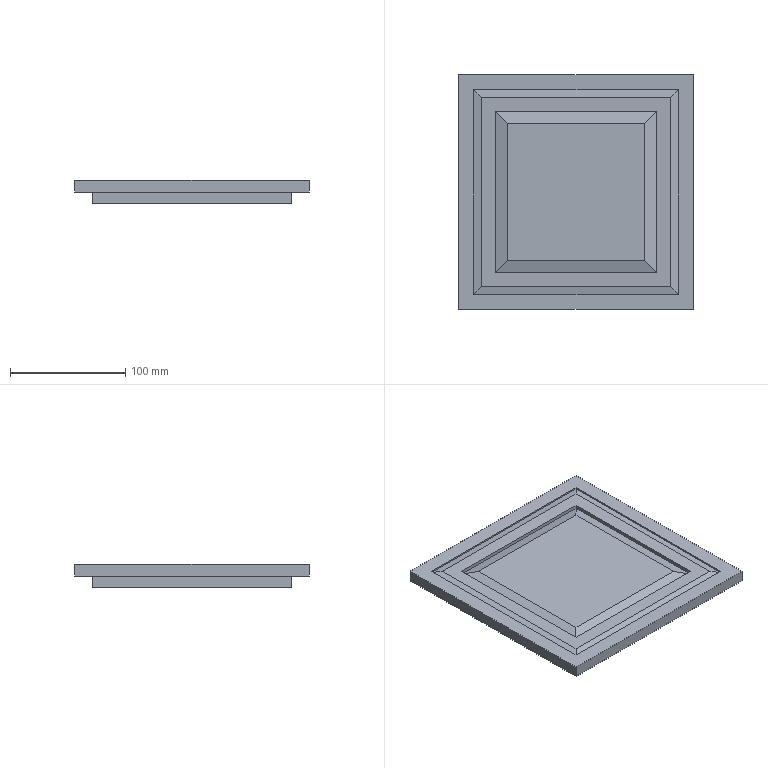Part | SolidWorks | features ICE 2, SweepCut 2, Extrusion 1 | 1 solid | 41 faces | box 204 x 204 x 20 mm | volume 703498 mm3 | plane 33 | cylinder 8 | commonest cylinder face diameters 5 x8
STEP:
#1=CARTESIAN_POINT('',(-89.5,-92.,3.));
#2=VERTEX_POINT('',#1);
#3=CARTESIAN_POINT('',(-94.5,-92.,3.));
#4=VERTEX_POINT('',#3);
#5=CARTESIAN_POINT('',(-92.,-92.,3.));
#6=DIRECTION('',(0.,0.,-1.));
#7=DIRECTION('',(-1.,0.,0.));
#8=AXIS2_PLACEMENT_3D('',#5,#6,#7);
#9=CIRCLE('',#8,2.5);
#10=EDGE_CURVE('',#2,#4,#9,.T.);
#11=ORIENTED_EDGE('',*,*,#10,.F.);
#12=CARTESIAN_POINT('',(-89.5,-92.,0.));
#13=VERTEX_POINT('',#12);
#14=CARTESIAN_POINT('',(-89.5,-92.,3.));
#15=DIRECTION('',(0.,0.,-1.));
#16=VECTOR('',#15,1000.);
#17=LINE('',#14,#16);
#18=EDGE_CURVE('',#2,#13,#17,.T.);
#19=ORIENTED_EDGE('',*,*,#18,.T.);
#20=CARTESIAN_POINT('',(-94.5,-92.,0.));
#21=VERTEX_POINT('',#20);
#22=CARTESIAN_POINT('',(-92.,-92.,0.));
#23=DIRECTION('',(0.,0.,-1.));
#24=DIRECTION('',(-1.,0.,0.));
#25=AXIS2_PLACEMENT_3D('',#22,#23,#24);
#26=CIRCLE('',#25,2.5);
#27=EDGE_CURVE('',#13,#21,#26,.T.);
#28=ORIENTED_EDGE('',*,*,#27,.T.);
#29=CARTESIAN_POINT('',(-94.5,-92.,3.));
#30=DIRECTION('',(0.,0.,-1.));
#31=VECTOR('',#30,1000.);
#32=LINE('',#29,#31);
#33=EDGE_CURVE('',#4,#21,#32,.T.);
#34=ORIENTED_EDGE('',*,*,#33,.F.);
#35=EDGE_LOOP('',(#11,#19,#28,#34));
#36=FACE_OUTER_BOUND('',#35,.T.);
#37=CARTESIAN_POINT('',(-92.,-92.,3.));
#38=DIRECTION('',(0.,0.,-1.));
#39=DIRECTION('',(-1.,0.,0.));
#40=AXIS2_PLACEMENT_3D('',#37,#38,#39);
#41=CYLINDRICAL_SURFACE('',#40,2.5);
#42=ADVANCED_FACE('',(#36),#41,.F.);
#43=CARTESIAN_POINT('',(94.5,-92.,3.));
#44=VERTEX_POINT('',#43);
#45=CARTESIAN_POINT('',(89.5,-92.,3.));
#46=VERTEX_POINT('',#45);
#47=CARTESIAN_POINT('',(92.,-92.,3.));
#48=DIRECTION('',(0.,0.,-1.));
#49=DIRECTION('',(-1.,0.,0.));
#50=AXIS2_PLACEMENT_3D('',#47,#48,#49);
#51=CIRCLE('',#50,2.5);
#52=EDGE_CURVE('',#44,#46,#51,.T.);
#53=ORIENTED_EDGE('',*,*,#52,.F.);
#54=CARTESIAN_POINT('',(94.5,-92.,0.));
#55=VERTEX_POINT('',#54);
#56=CARTESIAN_POINT('',(94.5,-92.,3.));
#57=DIRECTION('',(0.,0.,-1.));
#58=VECTOR('',#57,1000.);
#59=LINE('',#56,#58);
#60=EDGE_CURVE('',#44,#55,#59,.T.);
#61=ORIENTED_EDGE('',*,*,#60,.T.);
#62=CARTESIAN_POINT('',(89.5,-92.,0.));
#63=VERTEX_POINT('',#62);
#64=CARTESIAN_POINT('',(92.,-92.,0.));
#65=DIRECTION('',(0.,0.,-1.));
#66=DIRECTION('',(-1.,0.,0.));
#67=AXIS2_PLACEMENT_3D('',#64,#65,#66);
#68=CIRCLE('',#67,2.5);
#69=EDGE_CURVE('',#55,#63,#68,.T.);
#70=ORIENTED_EDGE('',*,*,#69,.T.);
#71=CARTESIAN_POINT('',(89.5,-92.,3.));
#72=DIRECTION('',(0.,0.,-1.));
#73=VECTOR('',#72,1000.);
#74=LINE('',#71,#73);
#75=EDGE_CURVE('',#46,#63,#74,.T.);
#76=ORIENTED_EDGE('',*,*,#75,.F.);
#77=EDGE_LOOP('',(#53,#61,#70,#76));
#78=FACE_OUTER_BOUND('',#77,.T.);
#79=CARTESIAN_POINT('',(92.,-92.,3.));
#80=DIRECTION('',(0.,0.,-1.));
#81=DIRECTION('',(-1.,0.,0.));
#82=AXIS2_PLACEMENT_3D('',#79,#80,#81);
#83=CYLINDRICAL_SURFACE('',#82,2.5);
#84=ADVANCED_FACE('',(#78),#83,.F.);
#85=CARTESIAN_POINT('',(-89.5,92.,3.));
#86=VERTEX_POINT('',#85);
#87=CARTESIAN_POINT('',(-94.5,92.,3.));
#88=VERTEX_POINT('',#87);
#89=CARTESIAN_POINT('',(-92.,92.,3.));
#90=DIRECTION('',(0.,0.,-1.));
#91=DIRECTION('',(-1.,0.,0.));
#92=AXIS2_PLACEMENT_3D('',#89,#90,#91);
#93=CIRCLE('',#92,2.5);
#94=EDGE_CURVE('',#86,#88,#93,.T.);
#95=ORIENTED_EDGE('',*,*,#94,.F.);
#96=CARTESIAN_POINT('',(-89.5,92.,0.));
#97=VERTEX_POINT('',#96);
#98=CARTESIAN_POINT('',(-89.5,92.,3.));
#99=DIRECTION('',(0.,0.,-1.));
#100=VECTOR('',#99,1000.);
#101=LINE('',#98,#100);
#102=EDGE_CURVE('',#86,#97,#101,.T.);
#103=ORIENTED_EDGE('',*,*,#102,.T.);
#104=CARTESIAN_POINT('',(-94.5,92.,0.));
#105=VERTEX_POINT('',#104);
#106=CARTESIAN_POINT('',(-92.,92.,0.));
#107=DIRECTION('',(0.,0.,-1.));
#108=DIRECTION('',(-1.,0.,0.));
#109=AXIS2_PLACEMENT_3D('',#106,#107,#108);
#110=CIRCLE('',#109,2.5);
#111=EDGE_CURVE('',#97,#105,#110,.T.);
#112=ORIENTED_EDGE('',*,*,#111,.T.);
#113=CARTESIAN_POINT('',(-94.5,92.,3.));
#114=DIRECTION('',(0.,0.,-1.));
#115=VECTOR('',#114,1000.);
#116=LINE('',#113,#115);
#117=EDGE_CURVE('',#88,#105,#116,.T.);
#118=ORIENTED_EDGE('',*,*,#117,.F.);
#119=EDGE_LOOP('',(#95,#103,#112,#118));
#120=FACE_OUTER_BOUND('',#119,.T.);
#121=CARTESIAN_POINT('',(-92.,92.,3.));
#122=DIRECTION('',(0.,0.,-1.));
#123=DIRECTION('',(-1.,0.,0.));
#124=AXIS2_PLACEMENT_3D('',#121,#122,#123);
#125=CYLINDRICAL_SURFACE('',#124,2.5);
#126=ADVANCED_FACE('',(#120),#125,.F.);
#127=CARTESIAN_POINT('',(94.5,92.,3.));
#128=VERTEX_POINT('',#127);
#129=CARTESIAN_POINT('',(89.5,92.,3.));
#130=VERTEX_POINT('',#129);
#131=CARTESIAN_POINT('',(92.,92.,3.));
#132=DIRECTION('',(0.,0.,-1.));
#133=DIRECTION('',(-1.,0.,0.));
#134=AXIS2_PLACEMENT_3D('',#131,#132,#133);
#135=CIRCLE('',#134,2.5);
#136=EDGE_CURVE('',#128,#130,#135,.T.);
#137=ORIENTED_EDGE('',*,*,#136,.F.);
#138=CARTESIAN_POINT('',(94.5,92.,0.));
#139=VERTEX_POINT('',#138);
#140=CARTESIAN_POINT('',(94.5,92.,3.));
#141=DIRECTION('',(0.,0.,-1.));
#142=VECTOR('',#141,1000.);
#143=LINE('',#140,#142);
#144=EDGE_CURVE('',#128,#139,#143,.T.);
#145=ORIENTED_EDGE('',*,*,#144,.T.);
#146=CARTESIAN_POINT('',(89.5,92.,0.));
#147=VERTEX_POINT('',#146);
#148=CARTESIAN_POINT('',(92.,92.,0.));
#149=DIRECTION('',(0.,0.,-1.));
#150=DIRECTION('',(-1.,0.,0.));
#151=AXIS2_PLACEMENT_3D('',#148,#149,#150);
#152=CIRCLE('',#151,2.5);
#153=EDGE_CURVE('',#139,#147,#152,.T.);
#154=ORIENTED_EDGE('',*,*,#153,.T.);
#155=CARTESIAN_POINT('',(89.5,92.,3.));
#156=DIRECTION('',(0.,0.,-1.));
#157=VECTOR('',#156,1000.);
#158=LINE('',#155,#157);
#159=EDGE_CURVE('',#130,#147,#158,.T.);
#160=ORIENTED_EDGE('',*,*,#159,.F.);
#161=EDGE_LOOP('',(#137,#145,#154,#160));
#162=FACE_OUTER_BOUND('',#161,.T.);
#163=CARTESIAN_POINT('',(92.,92.,3.));
#164=DIRECTION('',(0.,0.,-1.));
#165=DIRECTION('',(-1.,0.,0.));
#166=AXIS2_PLACEMENT_3D('',#163,#164,#165);
#167=CYLINDRICAL_SURFACE('',#166,2.5);
#168=ADVANCED_FACE('',(#162),#167,.F.);
#169=CARTESIAN_POINT('',(102.,-102.,0.));
#170=VERTEX_POINT('',#169);
#171=CARTESIAN_POINT('',(102.,102.,0.));
#172=VERTEX_POINT('',#171);
#173=CARTESIAN_POINT('',(102.,-102.,0.));
#174=DIRECTION('',(0.,1.,0.));
#175=VECTOR('',#174,1000.);
#176=LINE('',#173,#175);
#177=EDGE_CURVE('',#170,#172,#176,.T.);
#178=ORIENTED_EDGE('',*,*,#177,.F.);
#179=CARTESIAN_POINT('',(-102.,-102.,0.));
#180=VERTEX_POINT('',#179);
#181=CARTESIAN_POINT('',(-102.,-102.,0.));
#182=DIRECTION('',(1.,0.,0.));
#183=VECTOR('',#182,1000.);
#184=LINE('',#181,#183);
#185=EDGE_CURVE('',#180,#170,#184,.T.);
#186=ORIENTED_EDGE('',*,*,#185,.F.);
#187=CARTESIAN_POINT('',(-102.,102.,0.));
#188=VERTEX_POINT('',#187);
#189=CARTESIAN_POINT('',(-102.,-102.,0.));
#190=DIRECTION('',(0.,-1.,0.));
#191=VECTOR('',#190,1000.);
#192=LINE('',#189,#191);
#193=EDGE_CURVE('',#188,#180,#192,.T.);
#194=ORIENTED_EDGE('',*,*,#193,.F.);
#195=CARTESIAN_POINT('',(-102.,102.,0.));
#196=DIRECTION('',(-1.,0.,0.));
#197=VECTOR('',#196,1000.);
#198=LINE('',#195,#197);
#199=EDGE_CURVE('',#172,#188,#198,.T.);
#200=ORIENTED_EDGE('',*,*,#199,.F.);
#201=EDGE_LOOP('',(#178,#186,#194,#200));
#202=FACE_OUTER_BOUND('',#201,.T.);
#203=CARTESIAN_POINT('',(92.,92.,0.));
#204=DIRECTION('',(0.,0.,-1.));
#205=DIRECTION('',(-1.,0.,0.));
#206=AXIS2_PLACEMENT_3D('',#203,#204,#205);
#207=CIRCLE('',#206,2.5);
#208=EDGE_CURVE('',#147,#139,#207,.T.);
#209=ORIENTED_EDGE('',*,*,#208,.F.);
#210=ORIENTED_EDGE('',*,*,#153,.F.);
#211=EDGE_LOOP('',(#209,#210));
#212=FACE_BOUND('',#211,.T.);
#213=CARTESIAN_POINT('',(-92.,92.,0.));
#214=DIRECTION('',(0.,0.,-1.));
#215=DIRECTION('',(-1.,0.,0.));
#216=AXIS2_PLACEMENT_3D('',#213,#214,#215);
#217=CIRCLE('',#216,2.5);
#218=EDGE_CURVE('',#105,#97,#217,.T.);
#219=ORIENTED_EDGE('',*,*,#218,.F.);
#220=ORIENTED_EDGE('',*,*,#111,.F.);
#221=EDGE_LOOP('',(#219,#220));
#222=FACE_BOUND('',#221,.T.);
#223=CARTESIAN_POINT('',(92.,-92.,0.));
#224=DIRECTION('',(0.,0.,-1.));
#225=DIRECTION('',(-1.,0.,0.));
#226=AXIS2_PLACEMENT_3D('',#223,#224,#225);
#227=CIRCLE('',#226,2.5);
#228=EDGE_CURVE('',#63,#55,#227,.T.);
#229=ORIENTED_EDGE('',*,*,#228,.F.);
#230=ORIENTED_EDGE('',*,*,#69,.F.);
#231=EDGE_LOOP('',(#229,#230));
#232=FACE_BOUND('',#231,.T.);
#233=CARTESIAN_POINT('',(-92.,-92.,0.));
#234=DIRECTION('',(0.,0.,-1.));
#235=DIRECTION('',(-1.,0.,0.));
#236=AXIS2_PLACEMENT_3D('',#233,#234,#235);
#237=CIRCLE('',#236,2.5);
#238=EDGE_CURVE('',#21,#13,#237,.T.);
#239=ORIENTED_EDGE('',*,*,#238,.F.);
#240=ORIENTED_EDGE('',*,*,#27,.F.);
#241=EDGE_LOOP('',(#239,#240));
#242=FACE_BOUND('',#241,.T.);
#243=CARTESIAN_POINT('',(86.5,-86.5,0.));
#244=VERTEX_POINT('',#243);
#245=CARTESIAN_POINT('',(-86.5,-86.5,0.));
#246=VERTEX_POINT('',#245);
#247=CARTESIAN_POINT('',(86.5,-86.5,0.));
#248=DIRECTION('',(-1.,0.,0.));
#249=VECTOR('',#248,1000.);
#250=LINE('',#247,#249);
#251=EDGE_CURVE('',#244,#246,#250,.T.);
#252=ORIENTED_EDGE('',*,*,#251,.F.);
#253=CARTESIAN_POINT('',(86.5,86.5,0.));
#254=VERTEX_POINT('',#253);
#255=CARTESIAN_POINT('',(86.5,86.5,0.));
#256=DIRECTION('',(0.,-1.,0.));
#257=VECTOR('',#256,1000.);
#258=LINE('',#255,#257);
#259=EDGE_CURVE('',#254,#244,#258,.T.);
#260=ORIENTED_EDGE('',*,*,#259,.F.);
#261=CARTESIAN_POINT('',(-86.5,86.5,0.));
#262=VERTEX_POINT('',#261);
#263=CARTESIAN_POINT('',(86.5,86.5,0.));
#264=DIRECTION('',(1.,0.,0.));
#265=VECTOR('',#264,1000.);
#266=LINE('',#263,#265);
#267=EDGE_CURVE('',#262,#254,#266,.T.);
#268=ORIENTED_EDGE('',*,*,#267,.F.);
#269=CARTESIAN_POINT('',(-86.5,86.5,0.));
#270=DIRECTION('',(0.,1.,0.));
#271=VECTOR('',#270,1000.);
#272=LINE('',#269,#271);
#273=EDGE_CURVE('',#246,#262,#272,.T.);
#274=ORIENTED_EDGE('',*,*,#273,.F.);
#275=EDGE_LOOP('',(#252,#260,#268,#274));
#276=FACE_BOUND('',#275,.T.);
#277=CARTESIAN_POINT('',(0.,0.,0.));
#278=DIRECTION('',(0.,0.,-1.));
#279=DIRECTION('',(-1.,0.,0.));
#280=AXIS2_PLACEMENT_3D('',#277,#278,#279);
#281=PLANE('',#280);
#282=ADVANCED_FACE('',(#202,#212,#222,#232,#242,#276),#281,.T.);
#283=CARTESIAN_POINT('',(88.948,88.948,10.));
#284=VERTEX_POINT('',#283);
#285=CARTESIAN_POINT('',(88.948,-88.948,10.));
#286=VERTEX_POINT('',#285);
#287=CARTESIAN_POINT('',(88.948,88.948,10.));
#288=DIRECTION('',(0.,-1.,0.));
#289=VECTOR('',#288,1000.);
#290=LINE('',#287,#289);
#291=EDGE_CURVE('',#284,#286,#290,.T.);
#292=ORIENTED_EDGE('',*,*,#291,.T.);
#293=CARTESIAN_POINT('',(-88.948,-88.948,10.));
#294=VERTEX_POINT('',#293);
#295=CARTESIAN_POINT('',(88.948,-88.948,10.));
#296=DIRECTION('',(-1.,0.,0.));
#297=VECTOR('',#296,1000.);
#298=LINE('',#295,#297);
#299=EDGE_CURVE('',#286,#294,#298,.T.);
#300=ORIENTED_EDGE('',*,*,#299,.T.);
#301=CARTESIAN_POINT('',(-88.948,88.948,10.));
#302=VERTEX_POINT('',#301);
#303=CARTESIAN_POINT('',(-88.948,99.214,10.));
#304=DIRECTION('',(0.,-1.,0.));
#305=VECTOR('',#304,1000.);
#306=LINE('',#303,#305);
#307=EDGE_CURVE('',#302,#294,#306,.T.);
#308=ORIENTED_EDGE('',*,*,#307,.F.);
#309=CARTESIAN_POINT('',(-88.948,88.948,10.));
#310=DIRECTION('',(1.,0.,0.));
#311=VECTOR('',#310,1000.);
#312=LINE('',#309,#311);
#313=EDGE_CURVE('',#302,#284,#312,.T.);
#314=ORIENTED_EDGE('',*,*,#313,.T.);
#315=EDGE_LOOP('',(#292,#300,#308,#314));
#316=FACE_BOUND('',#315,.T.);
#317=CARTESIAN_POINT('',(102.,-102.,10.));
#318=VERTEX_POINT('',#317);
#319=CARTESIAN_POINT('',(102.,102.,10.));
#320=VERTEX_POINT('',#319);
#321=CARTESIAN_POINT('',(102.,-102.,10.));
#322=DIRECTION('',(0.,1.,0.));
#323=VECTOR('',#322,1000.);
#324=LINE('',#321,#323);
#325=EDGE_CURVE('',#318,#320,#324,.T.);
#326=ORIENTED_EDGE('',*,*,#325,.T.);
#327=CARTESIAN_POINT('',(-102.,102.,10.));
#328=VERTEX_POINT('',#327);
#329=CARTESIAN_POINT('',(-102.,102.,10.));
#330=DIRECTION('',(-1.,0.,0.));
#331=VECTOR('',#330,1000.);
#332=LINE('',#329,#331);
#333=EDGE_CURVE('',#320,#328,#332,.T.);
#334=ORIENTED_EDGE('',*,*,#333,.T.);
#335=CARTESIAN_POINT('',(-102.,-102.,10.));
#336=VERTEX_POINT('',#335);
#337=CARTESIAN_POINT('',(-102.,-102.,10.));
#338=DIRECTION('',(0.,-1.,0.));
#339=VECTOR('',#338,1000.);
#340=LINE('',#337,#339);
#341=EDGE_CURVE('',#328,#336,#340,.T.);
#342=ORIENTED_EDGE('',*,*,#341,.T.);
#343=CARTESIAN_POINT('',(-102.,-102.,10.));
#344=DIRECTION('',(1.,0.,0.));
#345=VECTOR('',#344,1000.);
#346=LINE('',#343,#345);
#347=EDGE_CURVE('',#336,#318,#346,.T.);
#348=ORIENTED_EDGE('',*,*,#347,.T.);
#349=EDGE_LOOP('',(#326,#334,#342,#348));
#350=FACE_OUTER_BOUND('',#349,.T.);
#351=CARTESIAN_POINT('',(0.,0.,10.));
#352=DIRECTION('',(0.,0.,-1.));
#353=DIRECTION('',(-1.,0.,0.));
#354=AXIS2_PLACEMENT_3D('',#351,#352,#353);
#355=PLANE('',#354);
#356=ADVANCED_FACE('',(#316,#350),#355,.F.);
#357=ORIENTED_EDGE('',*,*,#177,.T.);
#358=CARTESIAN_POINT('',(102.,102.,10.));
#359=DIRECTION('',(0.,0.,-1.));
#360=VECTOR('',#359,1000.);
#361=LINE('',#358,#360);
#362=EDGE_CURVE('',#320,#172,#361,.T.);
#363=ORIENTED_EDGE('',*,*,#362,.F.);
#364=ORIENTED_EDGE('',*,*,#325,.F.);
#365=CARTESIAN_POINT('',(102.,-102.,10.));
#366=DIRECTION('',(0.,0.,-1.));
#367=VECTOR('',#366,1000.);
#368=LINE('',#365,#367);
#369=EDGE_CURVE('',#318,#170,#368,.T.);
#370=ORIENTED_EDGE('',*,*,#369,.T.);
#371=EDGE_LOOP('',(#357,#363,#364,#370));
#372=FACE_OUTER_BOUND('',#371,.T.);
#373=CARTESIAN_POINT('',(102.,-102.,10.));
#374=DIRECTION('',(-1.,0.,0.));
#375=DIRECTION('',(0.,0.,1.));
#376=AXIS2_PLACEMENT_3D('',#373,#374,#375);
#377=PLANE('',#376);
#378=ADVANCED_FACE('',(#372),#377,.F.);
#379=ORIENTED_EDGE('',*,*,#199,.T.);
#380=CARTESIAN_POINT('',(-102.,102.,10.));
#381=DIRECTION('',(0.,0.,-1.));
#382=VECTOR('',#381,1000.);
#383=LINE('',#380,#382);
#384=EDGE_CURVE('',#328,#188,#383,.T.);
#385=ORIENTED_EDGE('',*,*,#384,.F.);
#386=ORIENTED_EDGE('',*,*,#333,.F.);
#387=ORIENTED_EDGE('',*,*,#362,.T.);
#388=EDGE_LOOP('',(#379,#385,#386,#387));
#389=FACE_OUTER_BOUND('',#388,.T.);
#390=CARTESIAN_POINT('',(-102.,102.,10.));
#391=DIRECTION('',(0.,-1.,0.));
#392=DIRECTION('',(0.,0.,-1.));
#393=AXIS2_PLACEMENT_3D('',#390,#391,#392);
#394=PLANE('',#393);
#395=ADVANCED_FACE('',(#389),#394,.F.);
#396=ORIENTED_EDGE('',*,*,#193,.T.);
#397=CARTESIAN_POINT('',(-102.,-102.,10.));
#398=DIRECTION('',(0.,0.,-1.));
#399=VECTOR('',#398,1000.);
#400=LINE('',#397,#399);
#401=EDGE_CURVE('',#336,#180,#400,.T.);
#402=ORIENTED_EDGE('',*,*,#401,.F.);
#403=ORIENTED_EDGE('',*,*,#341,.F.);
#404=ORIENTED_EDGE('',*,*,#384,.T.);
#405=EDGE_LOOP('',(#396,#402,#403,#404));
#406=FACE_OUTER_BOUND('',#405,.T.);
#407=CARTESIAN_POINT('',(-102.,-102.,10.));
#408=DIRECTION('',(1.,0.,0.));
#409=DIRECTION('',(0.,0.,-1.));
#410=AXIS2_PLACEMENT_3D('',#407,#408,#409);
#411=PLANE('',#410);
#412=ADVANCED_FACE('',(#406),#411,.F.);
#413=ORIENTED_EDGE('',*,*,#185,.T.);
#414=ORIENTED_EDGE('',*,*,#369,.F.);
#415=ORIENTED_EDGE('',*,*,#347,.F.);
#416=ORIENTED_EDGE('',*,*,#401,.T.);
#417=EDGE_LOOP('',(#413,#414,#415,#416));
#418=FACE_OUTER_BOUND('',#417,.T.);
#419=CARTESIAN_POINT('',(-102.,-102.,10.));
#420=DIRECTION('',(0.,1.,0.));
#421=DIRECTION('',(0.,0.,1.));
#422=AXIS2_PLACEMENT_3D('',#419,#420,#421);
#423=PLANE('',#422);
#424=ADVANCED_FACE('',(#418),#423,.F.);
#425=ORIENTED_EDGE('',*,*,#299,.F.);
#426=CARTESIAN_POINT('',(88.948,-88.948,8.705));
#427=VERTEX_POINT('',#426);
#428=CARTESIAN_POINT('',(88.948,-88.948,10.));
#429=DIRECTION('',(0.,0.,1.));
#430=VECTOR('',#429,1000.);
#431=LINE('',#428,#430);
#432=EDGE_CURVE('',#427,#286,#431,.T.);
#433=ORIENTED_EDGE('',*,*,#432,.F.);
#434=CARTESIAN_POINT('',(-88.948,-88.948,8.705));
#435=VERTEX_POINT('',#434);
#436=CARTESIAN_POINT('',(88.948,-88.948,8.705));
#437=DIRECTION('',(-1.,0.,0.));
#438=VECTOR('',#437,1000.);
#439=LINE('',#436,#438);
#440=EDGE_CURVE('',#427,#435,#439,.T.);
#441=ORIENTED_EDGE('',*,*,#440,.T.);
#442=CARTESIAN_POINT('',(-88.948,-88.948,10.));
#443=DIRECTION('',(0.,0.,-1.));
#444=VECTOR('',#443,1000.);
#445=LINE('',#442,#444);
#446=EDGE_CURVE('',#294,#435,#445,.T.);
#447=ORIENTED_EDGE('',*,*,#446,.F.);
#448=EDGE_LOOP('',(#425,#433,#441,#447));
#449=FACE_OUTER_BOUND('',#448,.T.);
#450=CARTESIAN_POINT('',(88.948,-88.948,10.));
#451=DIRECTION('',(0.,-1.,0.));
#452=DIRECTION('',(0.,0.,-1.));
#453=AXIS2_PLACEMENT_3D('',#450,#451,#452);
#454=PLANE('',#453);
#455=ADVANCED_FACE('',(#449),#454,.F.);
#456=ORIENTED_EDGE('',*,*,#440,.F.);
#457=CARTESIAN_POINT('',(82.271,-82.271,10.));
#458=VERTEX_POINT('',#457);
#459=CARTESIAN_POINT('',(0.032,-0.032,25.946));
#460=DIRECTION('',(0.7006,-0.7006,-0.1358));
#461=VECTOR('',#460,1000.);
#462=LINE('',#459,#461);
#463=EDGE_CURVE('',#458,#427,#462,.T.);
#464=ORIENTED_EDGE('',*,*,#463,.F.);
#465=CARTESIAN_POINT('',(-82.271,-82.271,10.));
#466=VERTEX_POINT('',#465);
#467=CARTESIAN_POINT('',(82.271,-82.271,10.));
#468=DIRECTION('',(-1.,0.,0.));
#469=VECTOR('',#468,1000.);
#470=LINE('',#467,#469);
#471=EDGE_CURVE('',#458,#466,#470,.T.);
#472=ORIENTED_EDGE('',*,*,#471,.T.);
#473=CARTESIAN_POINT('',(-0.0005904,-0.0005904,25.952));
#474=DIRECTION('',(0.7006,0.7006,0.1358));
#475=VECTOR('',#474,1000.);
#476=LINE('',#473,#475);
#477=EDGE_CURVE('',#435,#466,#476,.T.);
#478=ORIENTED_EDGE('',*,*,#477,.F.);
#479=EDGE_LOOP('',(#456,#464,#472,#478));
#480=FACE_OUTER_BOUND('',#479,.T.);
#481=CARTESIAN_POINT('',(0.032,-0.032,25.946));
#482=DIRECTION('',(0.,0.1904,-0.9817));
#483=DIRECTION('',(0.,0.9817,0.1904));
#484=AXIS2_PLACEMENT_3D('',#481,#482,#483);
#485=PLANE('',#484);
#486=ADVANCED_FACE('',(#480),#485,.F.);
#487=ORIENTED_EDGE('',*,*,#432,.T.);
#488=ORIENTED_EDGE('',*,*,#291,.F.);
#489=CARTESIAN_POINT('',(88.948,88.948,8.705));
#490=VERTEX_POINT('',#489);
#491=CARTESIAN_POINT('',(88.948,88.948,10.));
#492=DIRECTION('',(0.,0.,-1.));
#493=VECTOR('',#492,1000.);
#494=LINE('',#491,#493);
#495=EDGE_CURVE('',#284,#490,#494,.T.);
#496=ORIENTED_EDGE('',*,*,#495,.T.);
#497=CARTESIAN_POINT('',(88.948,88.948,8.705));
#498=DIRECTION('',(0.,-1.,0.));
#499=VECTOR('',#498,1000.);
#500=LINE('',#497,#499);
#501=EDGE_CURVE('',#490,#427,#500,.T.);
#502=ORIENTED_EDGE('',*,*,#501,.T.);
#503=EDGE_LOOP('',(#487,#488,#496,#502));
#504=FACE_OUTER_BOUND('',#503,.T.);
#505=CARTESIAN_POINT('',(88.948,88.948,10.));
#506=DIRECTION('',(-1.,0.,0.));
#507=DIRECTION('',(0.,0.,1.));
#508=AXIS2_PLACEMENT_3D('',#505,#506,#507);
#509=PLANE('',#508);
#510=ADVANCED_FACE('',(#504),#509,.T.);
#511=ORIENTED_EDGE('',*,*,#463,.T.);
#512=ORIENTED_EDGE('',*,*,#501,.F.);
#513=CARTESIAN_POINT('',(82.271,82.271,10.));
#514=VERTEX_POINT('',#513);
#515=CARTESIAN_POINT('',(1.734,1.734,25.616));
#516=DIRECTION('',(-0.7006,-0.7006,0.1358));
#517=VECTOR('',#516,1000.);
#518=LINE('',#515,#517);
#519=EDGE_CURVE('',#490,#514,#518,.T.);
#520=ORIENTED_EDGE('',*,*,#519,.T.);
#521=CARTESIAN_POINT('',(82.271,82.271,10.));
#522=DIRECTION('',(0.,-1.,0.));
#523=VECTOR('',#522,1000.);
#524=LINE('',#521,#523);
#525=EDGE_CURVE('',#514,#458,#524,.T.);
#526=ORIENTED_EDGE('',*,*,#525,.T.);
#527=EDGE_LOOP('',(#511,#512,#520,#526));
#528=FACE_OUTER_BOUND('',#527,.T.);
#529=CARTESIAN_POINT('',(1.734,1.734,25.616));
#530=DIRECTION('',(0.1904,0.,0.9817));
#531=DIRECTION('',(0.9817,0.,-0.1904));
#532=AXIS2_PLACEMENT_3D('',#529,#530,#531);
#533=PLANE('',#532);
#534=ADVANCED_FACE('',(#528),#533,.T.);
#535=ORIENTED_EDGE('',*,*,#313,.F.);
#536=CARTESIAN_POINT('',(-88.948,88.948,8.705));
#537=VERTEX_POINT('',#536);
#538=CARTESIAN_POINT('',(-88.948,88.948,10.));
#539=DIRECTION('',(0.,0.,1.));
#540=VECTOR('',#539,1000.);
#541=LINE('',#538,#540);
#542=EDGE_CURVE('',#537,#302,#541,.T.);
#543=ORIENTED_EDGE('',*,*,#542,.F.);
#544=CARTESIAN_POINT('',(-88.948,88.948,8.705));
#545=DIRECTION('',(1.,0.,0.));
#546=VECTOR('',#545,1000.);
#547=LINE('',#544,#546);
#548=EDGE_CURVE('',#537,#490,#547,.T.);
#549=ORIENTED_EDGE('',*,*,#548,.T.);
#550=ORIENTED_EDGE('',*,*,#495,.F.);
#551=EDGE_LOOP('',(#535,#543,#549,#550));
#552=FACE_OUTER_BOUND('',#551,.T.);
#553=CARTESIAN_POINT('',(-88.948,88.948,10.));
#554=DIRECTION('',(0.,1.,0.));
#555=DIRECTION('',(0.,0.,1.));
#556=AXIS2_PLACEMENT_3D('',#553,#554,#555);
#557=PLANE('',#556);
#558=ADVANCED_FACE('',(#552),#557,.F.);
#559=ORIENTED_EDGE('',*,*,#548,.F.);
#560=CARTESIAN_POINT('',(-82.271,82.271,10.));
#561=VERTEX_POINT('',#560);
#562=CARTESIAN_POINT('',(-93.986,93.986,7.728));
#563=DIRECTION('',(-0.7006,0.7006,-0.1358));
#564=VECTOR('',#563,1000.);
#565=LINE('',#562,#564);
#566=EDGE_CURVE('',#561,#537,#565,.T.);
#567=ORIENTED_EDGE('',*,*,#566,.F.);
#568=CARTESIAN_POINT('',(-82.271,82.271,10.));
#569=DIRECTION('',(1.,0.,0.));
#570=VECTOR('',#569,1000.);
#571=LINE('',#568,#570);
#572=EDGE_CURVE('',#561,#514,#571,.T.);
#573=ORIENTED_EDGE('',*,*,#572,.T.);
#574=ORIENTED_EDGE('',*,*,#519,.F.);
#575=EDGE_LOOP('',(#559,#567,#573,#574));
#576=FACE_OUTER_BOUND('',#575,.T.);
#577=CARTESIAN_POINT('',(-93.986,93.986,7.728));
#578=DIRECTION('',(0.,-0.1904,-0.9817));
#579=DIRECTION('',(0.,0.9817,-0.1904));
#580=AXIS2_PLACEMENT_3D('',#577,#578,#579);
#581=PLANE('',#580);
#582=ADVANCED_FACE('',(#576),#581,.F.);
#583=ORIENTED_EDGE('',*,*,#542,.T.);
#584=ORIENTED_EDGE('',*,*,#307,.T.);
#585=ORIENTED_EDGE('',*,*,#446,.T.);
#586=CARTESIAN_POINT('',(-88.948,99.214,8.705));
#587=DIRECTION('',(0.,-1.,0.));
#588=VECTOR('',#587,1000.);
#589=LINE('',#586,#588);
#590=EDGE_CURVE('',#537,#435,#589,.T.);
#591=ORIENTED_EDGE('',*,*,#590,.F.);
#592=EDGE_LOOP('',(#583,#584,#585,#591));
#593=FACE_OUTER_BOUND('',#592,.T.);
#594=CARTESIAN_POINT('',(-88.948,99.214,10.));
#595=DIRECTION('',(1.,0.,0.));
#596=DIRECTION('',(0.,0.,-1.));
#597=AXIS2_PLACEMENT_3D('',#594,#595,#596);
#598=PLANE('',#597);
#599=ADVANCED_FACE('',(#593),#598,.T.);
#600=ORIENTED_EDGE('',*,*,#566,.T.);
#601=ORIENTED_EDGE('',*,*,#590,.T.);
#602=ORIENTED_EDGE('',*,*,#477,.T.);
#603=CARTESIAN_POINT('',(-82.271,99.214,10.));
#604=DIRECTION('',(0.,-1.,0.));
#605=VECTOR('',#604,1000.);
#606=LINE('',#603,#605);
#607=EDGE_CURVE('',#561,#466,#606,.T.);
#608=ORIENTED_EDGE('',*,*,#607,.F.);
#609=EDGE_LOOP('',(#600,#601,#602,#608));
#610=FACE_OUTER_BOUND('',#609,.T.);
#611=CARTESIAN_POINT('',(-88.948,99.214,8.705));
#612=DIRECTION('',(-0.1904,0.,0.9817));
#613=DIRECTION('',(0.9817,0.,0.1904));
#614=AXIS2_PLACEMENT_3D('',#611,#612,#613);
#615=PLANE('',#614);
#616=ADVANCED_FACE('',(#610),#615,.T.);
#617=CARTESIAN_POINT('',(70.049,70.049,10.));
#618=VERTEX_POINT('',#617);
#619=CARTESIAN_POINT('',(70.049,-70.049,10.));
#620=VERTEX_POINT('',#619);
#621=CARTESIAN_POINT('',(70.049,70.049,10.));
#622=DIRECTION('',(0.,-1.,0.));
#623=VECTOR('',#622,1000.);
#624=LINE('',#621,#623);
#625=EDGE_CURVE('',#618,#620,#624,.T.);
#626=ORIENTED_EDGE('',*,*,#625,.T.);
#627=CARTESIAN_POINT('',(-70.049,-70.049,10.));
#628=VERTEX_POINT('',#627);
#629=CARTESIAN_POINT('',(70.049,-70.049,10.));
#630=DIRECTION('',(-1.,0.,0.));
#631=VECTOR('',#630,1000.);
#632=LINE('',#629,#631);
#633=EDGE_CURVE('',#620,#628,#632,.T.);
#634=ORIENTED_EDGE('',*,*,#633,.T.);
#635=CARTESIAN_POINT('',(-70.049,70.049,10.));
#636=VERTEX_POINT('',#635);
#637=CARTESIAN_POINT('',(-70.049,86.63,10.));
#638=DIRECTION('',(0.,-1.,0.));
#639=VECTOR('',#638,1000.);
#640=LINE('',#637,#639);
#641=EDGE_CURVE('',#636,#628,#640,.T.);
#642=ORIENTED_EDGE('',*,*,#641,.F.);
#643=CARTESIAN_POINT('',(-70.049,70.049,10.));
#644=DIRECTION('',(1.,0.,0.));
#645=VECTOR('',#644,1000.);
#646=LINE('',#643,#645);
#647=EDGE_CURVE('',#636,#618,#646,.T.);
#648=ORIENTED_EDGE('',*,*,#647,.T.);
#649=EDGE_LOOP('',(#626,#634,#642,#648));
#650=FACE_BOUND('',#649,.T.);
#651=ORIENTED_EDGE('',*,*,#607,.T.);
#652=ORIENTED_EDGE('',*,*,#471,.F.);
#653=ORIENTED_EDGE('',*,*,#525,.F.);
#654=ORIENTED_EDGE('',*,*,#572,.F.);
#655=EDGE_LOOP('',(#651,#652,#653,#654));
#656=FACE_OUTER_BOUND('',#655,.T.);
#657=CARTESIAN_POINT('',(0.,0.,10.));
#658=DIRECTION('',(0.,0.,-1.));
#659=DIRECTION('',(-1.,0.,0.));
#660=AXIS2_PLACEMENT_3D('',#657,#658,#659);
#661=PLANE('',#660);
#662=ADVANCED_FACE('',(#650,#656),#661,.F.);
#663=ORIENTED_EDGE('',*,*,#633,.F.);
#664=CARTESIAN_POINT('',(70.049,-70.049,6.864));
#665=VERTEX_POINT('',#664);
#666=CARTESIAN_POINT('',(70.049,-70.049,10.));
#667=DIRECTION('',(0.,0.,1.));
#668=VECTOR('',#667,1000.);
#669=LINE('',#666,#668);
#670=EDGE_CURVE('',#665,#620,#669,.T.);
#671=ORIENTED_EDGE('',*,*,#670,.F.);
#672=CARTESIAN_POINT('',(-70.049,-70.049,6.864));
#673=VERTEX_POINT('',#672);
#674=CARTESIAN_POINT('',(70.049,-70.049,6.864));
#675=DIRECTION('',(-1.,0.,0.));
#676=VECTOR('',#675,1000.);
#677=LINE('',#674,#676);
#678=EDGE_CURVE('',#665,#673,#677,.T.);
#679=ORIENTED_EDGE('',*,*,#678,.T.);
#680=CARTESIAN_POINT('',(-70.049,-70.049,10.));
#681=DIRECTION('',(0.,0.,-1.));
#682=VECTOR('',#681,1000.);
#683=LINE('',#680,#682);
#684=EDGE_CURVE('',#628,#673,#683,.T.);
#685=ORIENTED_EDGE('',*,*,#684,.F.);
#686=EDGE_LOOP('',(#663,#671,#679,#685));
#687=FACE_OUTER_BOUND('',#686,.T.);
#688=CARTESIAN_POINT('',(70.049,-70.049,10.));
#689=DIRECTION('',(0.,-1.,0.));
#690=DIRECTION('',(0.,0.,-1.));
#691=AXIS2_PLACEMENT_3D('',#688,#689,#690);
#692=PLANE('',#691);
#693=ADVANCED_FACE('',(#687),#692,.F.);
#694=ORIENTED_EDGE('',*,*,#678,.F.);
#695=CARTESIAN_POINT('',(59.609,-59.609,10.));
#696=VERTEX_POINT('',#695);
#697=CARTESIAN_POINT('',(0.1453,-0.1453,27.861));
#698=DIRECTION('',(0.6917,-0.6917,-0.2078));
#699=VECTOR('',#698,1000.);
#700=LINE('',#697,#699);
#701=EDGE_CURVE('',#696,#665,#700,.T.);
#702=ORIENTED_EDGE('',*,*,#701,.F.);
#703=CARTESIAN_POINT('',(-59.609,-59.609,10.));
#704=VERTEX_POINT('',#703);
#705=CARTESIAN_POINT('',(59.609,-59.609,10.));
#706=DIRECTION('',(-1.,0.,0.));
#707=VECTOR('',#706,1000.);
#708=LINE('',#705,#707);
#709=EDGE_CURVE('',#696,#704,#708,.T.);
#710=ORIENTED_EDGE('',*,*,#709,.T.);
#711=CARTESIAN_POINT('',(-0.006271,-0.006271,27.902));
#712=DIRECTION('',(0.6917,0.6917,0.2078));
#713=VECTOR('',#712,1000.);
#714=LINE('',#711,#713);
#715=EDGE_CURVE('',#673,#704,#714,.T.);
#716=ORIENTED_EDGE('',*,*,#715,.F.);
#717=EDGE_LOOP('',(#694,#702,#710,#716));
#718=FACE_OUTER_BOUND('',#717,.T.);
#719=CARTESIAN_POINT('',(0.1453,-0.1453,27.861));
#720=DIRECTION('',(0.,0.2877,-0.9577));
#721=DIRECTION('',(0.,0.9577,0.2877));
#722=AXIS2_PLACEMENT_3D('',#719,#720,#721);
#723=PLANE('',#722);
#724=ADVANCED_FACE('',(#718),#723,.F.);
#725=ORIENTED_EDGE('',*,*,#670,.T.);
#726=ORIENTED_EDGE('',*,*,#625,.F.);
#727=CARTESIAN_POINT('',(70.049,70.049,6.864));
#728=VERTEX_POINT('',#727);
#729=CARTESIAN_POINT('',(70.049,70.049,10.));
#730=DIRECTION('',(0.,0.,-1.));
#731=VECTOR('',#730,1000.);
#732=LINE('',#729,#731);
#733=EDGE_CURVE('',#618,#728,#732,.T.);
#734=ORIENTED_EDGE('',*,*,#733,.T.);
#735=CARTESIAN_POINT('',(70.049,70.049,6.864));
#736=DIRECTION('',(0.,-1.,0.));
#737=VECTOR('',#736,1000.);
#738=LINE('',#735,#737);
#739=EDGE_CURVE('',#728,#665,#738,.T.);
#740=ORIENTED_EDGE('',*,*,#739,.T.);
#741=EDGE_LOOP('',(#725,#726,#734,#740));
#742=FACE_OUTER_BOUND('',#741,.T.);
#743=CARTESIAN_POINT('',(70.049,70.049,10.));
#744=DIRECTION('',(-1.,0.,0.));
#745=DIRECTION('',(0.,0.,1.));
#746=AXIS2_PLACEMENT_3D('',#743,#744,#745);
#747=PLANE('',#746);
#748=ADVANCED_FACE('',(#742),#747,.T.);
#749=ORIENTED_EDGE('',*,*,#701,.T.);
#750=ORIENTED_EDGE('',*,*,#739,.F.);
#751=CARTESIAN_POINT('',(59.609,59.609,10.));
#752=VERTEX_POINT('',#751);
#753=CARTESIAN_POINT('',(3.366,3.366,26.893));
#754=DIRECTION('',(-0.6917,-0.6917,0.2078));
#755=VECTOR('',#754,1000.);
#756=LINE('',#753,#755);
#757=EDGE_CURVE('',#728,#752,#756,.T.);
#758=ORIENTED_EDGE('',*,*,#757,.T.);
#759=CARTESIAN_POINT('',(59.609,59.609,10.));
#760=DIRECTION('',(0.,-1.,0.));
#761=VECTOR('',#760,1000.);
#762=LINE('',#759,#761);
#763=EDGE_CURVE('',#752,#696,#762,.T.);
#764=ORIENTED_EDGE('',*,*,#763,.T.);
#765=EDGE_LOOP('',(#749,#750,#758,#764));
#766=FACE_OUTER_BOUND('',#765,.T.);
#767=CARTESIAN_POINT('',(3.366,3.366,26.893));
#768=DIRECTION('',(0.2877,0.,0.9577));
#769=DIRECTION('',(0.9577,0.,-0.2877));
#770=AXIS2_PLACEMENT_3D('',#767,#768,#769);
#771=PLANE('',#770);
#772=ADVANCED_FACE('',(#766),#771,.T.);
#773=CARTESIAN_POINT('',(-70.049,70.049,6.864));
#774=VERTEX_POINT('',#773);
#775=CARTESIAN_POINT('',(-70.049,70.049,6.864));
#776=DIRECTION('',(1.,0.,0.));
#777=VECTOR('',#776,1000.);
#778=LINE('',#775,#777);
#779=EDGE_CURVE('',#774,#728,#778,.T.);
#780=ORIENTED_EDGE('',*,*,#779,.F.);
#781=CARTESIAN_POINT('',(-59.609,59.609,10.));
#782=VERTEX_POINT('',#781);
#783=CARTESIAN_POINT('',(-77.982,77.982,4.481));
#784=DIRECTION('',(-0.6917,0.6917,-0.2078));
#785=VECTOR('',#784,1000.);
#786=LINE('',#783,#785);
#787=EDGE_CURVE('',#782,#774,#786,.T.);
#788=ORIENTED_EDGE('',*,*,#787,.F.);
#789=CARTESIAN_POINT('',(-59.609,59.609,10.));
#790=DIRECTION('',(1.,0.,0.));
#791=VECTOR('',#790,1000.);
#792=LINE('',#789,#791);
#793=EDGE_CURVE('',#782,#752,#792,.T.);
#794=ORIENTED_EDGE('',*,*,#793,.T.);
#795=ORIENTED_EDGE('',*,*,#757,.F.);
#796=EDGE_LOOP('',(#780,#788,#794,#795));
#797=FACE_OUTER_BOUND('',#796,.T.);
#798=CARTESIAN_POINT('',(-77.982,77.982,4.481));
#799=DIRECTION('',(0.,-0.2877,-0.9577));
#800=DIRECTION('',(0.,0.9577,-0.2877));
#801=AXIS2_PLACEMENT_3D('',#798,#799,#800);
#802=PLANE('',#801);
#803=ADVANCED_FACE('',(#797),#802,.F.);
#804=ORIENTED_EDGE('',*,*,#647,.F.);
#805=CARTESIAN_POINT('',(-70.049,70.049,10.));
#806=DIRECTION('',(0.,0.,1.));
#807=VECTOR('',#806,1000.);
#808=LINE('',#805,#807);
#809=EDGE_CURVE('',#774,#636,#808,.T.);
#810=ORIENTED_EDGE('',*,*,#809,.F.);
#811=ORIENTED_EDGE('',*,*,#779,.T.);
#812=ORIENTED_EDGE('',*,*,#733,.F.);
#813=EDGE_LOOP('',(#804,#810,#811,#812));
#814=FACE_OUTER_BOUND('',#813,.T.);
#815=CARTESIAN_POINT('',(-70.049,70.049,10.));
#816=DIRECTION('',(0.,1.,0.));
#817=DIRECTION('',(0.,0.,1.));
#818=AXIS2_PLACEMENT_3D('',#815,#816,#817);
#819=PLANE('',#818);
#820=ADVANCED_FACE('',(#814),#819,.F.);
#821=ORIENTED_EDGE('',*,*,#787,.T.);
#822=CARTESIAN_POINT('',(-70.049,86.63,6.864));
#823=DIRECTION('',(0.,-1.,0.));
#824=VECTOR('',#823,1000.);
#825=LINE('',#822,#824);
#826=EDGE_CURVE('',#774,#673,#825,.T.);
#827=ORIENTED_EDGE('',*,*,#826,.T.);
#828=ORIENTED_EDGE('',*,*,#715,.T.);
#829=CARTESIAN_POINT('',(-59.609,86.63,10.));
#830=DIRECTION('',(0.,-1.,0.));
#831=VECTOR('',#830,1000.);
#832=LINE('',#829,#831);
#833=EDGE_CURVE('',#782,#704,#832,.T.);
#834=ORIENTED_EDGE('',*,*,#833,.F.);
#835=EDGE_LOOP('',(#821,#827,#828,#834));
#836=FACE_OUTER_BOUND('',#835,.T.);
#837=CARTESIAN_POINT('',(-70.049,86.63,6.864));
#838=DIRECTION('',(-0.2877,0.,0.9577));
#839=DIRECTION('',(0.9577,0.,0.2877));
#840=AXIS2_PLACEMENT_3D('',#837,#838,#839);
#841=PLANE('',#840);
#842=ADVANCED_FACE('',(#836),#841,.T.);
#843=ORIENTED_EDGE('',*,*,#809,.T.);
#844=ORIENTED_EDGE('',*,*,#641,.T.);
#845=ORIENTED_EDGE('',*,*,#684,.T.);
#846=ORIENTED_EDGE('',*,*,#826,.F.);
#847=EDGE_LOOP('',(#843,#844,#845,#846));
#848=FACE_OUTER_BOUND('',#847,.T.);
#849=CARTESIAN_POINT('',(-70.049,86.63,10.));
#850=DIRECTION('',(1.,0.,0.));
#851=DIRECTION('',(0.,0.,-1.));
#852=AXIS2_PLACEMENT_3D('',#849,#850,#851);
#853=PLANE('',#852);
#854=ADVANCED_FACE('',(#848),#853,.T.);
#855=ORIENTED_EDGE('',*,*,#833,.T.);
#856=ORIENTED_EDGE('',*,*,#709,.F.);
#857=ORIENTED_EDGE('',*,*,#763,.F.);
#858=ORIENTED_EDGE('',*,*,#793,.F.);
#859=EDGE_LOOP('',(#855,#856,#857,#858));
#860=FACE_OUTER_BOUND('',#859,.T.);
#861=CARTESIAN_POINT('',(0.,0.,10.));
#862=DIRECTION('',(0.,0.,-1.));
#863=DIRECTION('',(-1.,0.,0.));
#864=AXIS2_PLACEMENT_3D('',#861,#862,#863);
#865=PLANE('',#864);
#866=ADVANCED_FACE('',(#860),#865,.F.);
#867=ORIENTED_EDGE('',*,*,#144,.F.);
#868=CARTESIAN_POINT('',(92.,92.,3.));
#869=DIRECTION('',(0.,0.,-1.));
#870=DIRECTION('',(-1.,0.,0.));
#871=AXIS2_PLACEMENT_3D('',#868,#869,#870);
#872=CIRCLE('',#871,2.5);
#873=EDGE_CURVE('',#130,#128,#872,.T.);
#874=ORIENTED_EDGE('',*,*,#873,.F.);
#875=ORIENTED_EDGE('',*,*,#159,.T.);
#876=ORIENTED_EDGE('',*,*,#208,.T.);
#877=EDGE_LOOP('',(#867,#874,#875,#876));
#878=FACE_OUTER_BOUND('',#877,.T.);
#879=CARTESIAN_POINT('',(92.,92.,3.));
#880=DIRECTION('',(0.,0.,-1.));
#881=DIRECTION('',(-1.,0.,0.));
#882=AXIS2_PLACEMENT_3D('',#879,#880,#881);
#883=CYLINDRICAL_SURFACE('',#882,2.5);
#884=ADVANCED_FACE('',(#878),#883,.F.);
#885=ORIENTED_EDGE('',*,*,#873,.T.);
#886=ORIENTED_EDGE('',*,*,#136,.T.);
#887=EDGE_LOOP('',(#885,#886));
#888=FACE_OUTER_BOUND('',#887,.T.);
#889=CARTESIAN_POINT('',(92.,92.,3.));
#890=DIRECTION('',(0.,0.,-1.));
#891=DIRECTION('',(-1.,0.,0.));
#892=AXIS2_PLACEMENT_3D('',#889,#890,#891);
#893=PLANE('',#892);
#894=ADVANCED_FACE('',(#888),#893,.T.);
#895=ORIENTED_EDGE('',*,*,#102,.F.);
#896=CARTESIAN_POINT('',(-92.,92.,3.));
#897=DIRECTION('',(0.,0.,-1.));
#898=DIRECTION('',(-1.,0.,0.));
#899=AXIS2_PLACEMENT_3D('',#896,#897,#898);
#900=CIRCLE('',#899,2.5);
#901=EDGE_CURVE('',#88,#86,#900,.T.);
#902=ORIENTED_EDGE('',*,*,#901,.F.);
#903=ORIENTED_EDGE('',*,*,#117,.T.);
#904=ORIENTED_EDGE('',*,*,#218,.T.);
#905=EDGE_LOOP('',(#895,#902,#903,#904));
#906=FACE_OUTER_BOUND('',#905,.T.);
#907=CARTESIAN_POINT('',(-92.,92.,3.));
#908=DIRECTION('',(0.,0.,-1.));
#909=DIRECTION('',(-1.,0.,0.));
#910=AXIS2_PLACEMENT_3D('',#907,#908,#909);
#911=CYLINDRICAL_SURFACE('',#910,2.5);
#912=ADVANCED_FACE('',(#906),#911,.F.);
#913=ORIENTED_EDGE('',*,*,#901,.T.);
#914=ORIENTED_EDGE('',*,*,#94,.T.);
#915=EDGE_LOOP('',(#913,#914));
#916=FACE_OUTER_BOUND('',#915,.T.);
#917=CARTESIAN_POINT('',(-92.,92.,3.));
#918=DIRECTION('',(0.,0.,-1.));
#919=DIRECTION('',(-1.,0.,0.));
#920=AXIS2_PLACEMENT_3D('',#917,#918,#919);
#921=PLANE('',#920);
#922=ADVANCED_FACE('',(#916),#921,.T.);
#923=ORIENTED_EDGE('',*,*,#60,.F.);
#924=CARTESIAN_POINT('',(92.,-92.,3.));
#925=DIRECTION('',(0.,0.,-1.));
#926=DIRECTION('',(-1.,0.,0.));
#927=AXIS2_PLACEMENT_3D('',#924,#925,#926);
#928=CIRCLE('',#927,2.5);
#929=EDGE_CURVE('',#46,#44,#928,.T.);
#930=ORIENTED_EDGE('',*,*,#929,.F.);
#931=ORIENTED_EDGE('',*,*,#75,.T.);
#932=ORIENTED_EDGE('',*,*,#228,.T.);
#933=EDGE_LOOP('',(#923,#930,#931,#932));
#934=FACE_OUTER_BOUND('',#933,.T.);
#935=CARTESIAN_POINT('',(92.,-92.,3.));
#936=DIRECTION('',(0.,0.,-1.));
#937=DIRECTION('',(-1.,0.,0.));
#938=AXIS2_PLACEMENT_3D('',#935,#936,#937);
#939=CYLINDRICAL_SURFACE('',#938,2.5);
#940=ADVANCED_FACE('',(#934),#939,.F.);
#941=ORIENTED_EDGE('',*,*,#929,.T.);
#942=ORIENTED_EDGE('',*,*,#52,.T.);
#943=EDGE_LOOP('',(#941,#942));
#944=FACE_OUTER_BOUND('',#943,.T.);
#945=CARTESIAN_POINT('',(92.,-92.,3.));
#946=DIRECTION('',(0.,0.,-1.));
#947=DIRECTION('',(-1.,0.,0.));
#948=AXIS2_PLACEMENT_3D('',#945,#946,#947);
#949=PLANE('',#948);
#950=ADVANCED_FACE('',(#944),#949,.T.);
#951=ORIENTED_EDGE('',*,*,#18,.F.);
#952=CARTESIAN_POINT('',(-92.,-92.,3.));
#953=DIRECTION('',(0.,0.,-1.));
#954=DIRECTION('',(-1.,0.,0.));
#955=AXIS2_PLACEMENT_3D('',#952,#953,#954);
#956=CIRCLE('',#955,2.5);
#957=EDGE_CURVE('',#4,#2,#956,.T.);
#958=ORIENTED_EDGE('',*,*,#957,.F.);
#959=ORIENTED_EDGE('',*,*,#33,.T.);
#960=ORIENTED_EDGE('',*,*,#238,.T.);
#961=EDGE_LOOP('',(#951,#958,#959,#960));
#962=FACE_OUTER_BOUND('',#961,.T.);
#963=CARTESIAN_POINT('',(-92.,-92.,3.));
#964=DIRECTION('',(0.,0.,-1.));
#965=DIRECTION('',(-1.,0.,0.));
#966=AXIS2_PLACEMENT_3D('',#963,#964,#965);
#967=CYLINDRICAL_SURFACE('',#966,2.5);
#968=ADVANCED_FACE('',(#962),#967,.F.);
#969=ORIENTED_EDGE('',*,*,#957,.T.);
#970=ORIENTED_EDGE('',*,*,#10,.T.);
#971=EDGE_LOOP('',(#969,#970));
#972=FACE_OUTER_BOUND('',#971,.T.);
#973=CARTESIAN_POINT('',(-92.,-92.,3.));
#974=DIRECTION('',(0.,0.,-1.));
#975=DIRECTION('',(-1.,0.,0.));
#976=AXIS2_PLACEMENT_3D('',#973,#974,#975);
#977=PLANE('',#976);
#978=ADVANCED_FACE('',(#972),#977,.T.);
#979=ORIENTED_EDGE('',*,*,#259,.T.);
#980=CARTESIAN_POINT('',(86.5,-86.5,-10.));
#981=VERTEX_POINT('',#980);
#982=CARTESIAN_POINT('',(86.5,-86.5,-10.));
#983=DIRECTION('',(0.,0.,1.));
#984=VECTOR('',#983,1000.);
#985=LINE('',#982,#984);
#986=EDGE_CURVE('',#981,#244,#985,.T.);
#987=ORIENTED_EDGE('',*,*,#986,.F.);
#988=CARTESIAN_POINT('',(86.5,86.5,-10.));
#989=VERTEX_POINT('',#988);
#990=CARTESIAN_POINT('',(86.5,86.5,-10.));
#991=DIRECTION('',(0.,-1.,0.));
#992=VECTOR('',#991,1000.);
#993=LINE('',#990,#992);
#994=EDGE_CURVE('',#989,#981,#993,.T.);
#995=ORIENTED_EDGE('',*,*,#994,.F.);
#996=CARTESIAN_POINT('',(86.5,86.5,-10.));
#997=DIRECTION('',(0.,0.,1.));
#998=VECTOR('',#997,1000.);
#999=LINE('',#996,#998);
#1000=EDGE_CURVE('',#989,#254,#999,.T.);
#1001=ORIENTED_EDGE('',*,*,#1000,.T.);
#1002=EDGE_LOOP('',(#979,#987,#995,#1001));
#1003=FACE_OUTER_BOUND('',#1002,.T.);
#1004=CARTESIAN_POINT('',(86.5,86.5,-10.));
#1005=DIRECTION('',(-1.,0.,0.));
#1006=DIRECTION('',(0.,-1.,0.));
#1007=AXIS2_PLACEMENT_3D('',#1004,#1005,#1006);
#1008=PLANE('',#1007);
#1009=ADVANCED_FACE('',(#1003),#1008,.F.);
#1010=ORIENTED_EDGE('',*,*,#251,.T.);
#1011=CARTESIAN_POINT('',(-86.5,-86.5,-10.));
#1012=VERTEX_POINT('',#1011);
#1013=CARTESIAN_POINT('',(-86.5,-86.5,-10.));
#1014=DIRECTION('',(0.,0.,1.));
#1015=VECTOR('',#1014,1000.);
#1016=LINE('',#1013,#1015);
#1017=EDGE_CURVE('',#1012,#246,#1016,.T.);
#1018=ORIENTED_EDGE('',*,*,#1017,.F.);
#1019=CARTESIAN_POINT('',(86.5,-86.5,-10.));
#1020=DIRECTION('',(-1.,0.,0.));
#1021=VECTOR('',#1020,1000.);
#1022=LINE('',#1019,#1021);
#1023=EDGE_CURVE('',#981,#1012,#1022,.T.);
#1024=ORIENTED_EDGE('',*,*,#1023,.F.);
#1025=ORIENTED_EDGE('',*,*,#986,.T.);
#1026=EDGE_LOOP('',(#1010,#1018,#1024,#1025));
#1027=FACE_OUTER_BOUND('',#1026,.T.);
#1028=CARTESIAN_POINT('',(86.5,-86.5,-10.));
#1029=DIRECTION('',(0.,1.,0.));
#1030=DIRECTION('',(-1.,0.,0.));
#1031=AXIS2_PLACEMENT_3D('',#1028,#1029,#1030);
#1032=PLANE('',#1031);
#1033=ADVANCED_FACE('',(#1027),#1032,.F.);
#1034=ORIENTED_EDGE('',*,*,#273,.T.);
#1035=CARTESIAN_POINT('',(-86.5,86.5,-10.));
#1036=VERTEX_POINT('',#1035);
#1037=CARTESIAN_POINT('',(-86.5,86.5,-10.));
#1038=DIRECTION('',(0.,0.,1.));
#1039=VECTOR('',#1038,1000.);
#1040=LINE('',#1037,#1039);
#1041=EDGE_CURVE('',#1036,#262,#1040,.T.);
#1042=ORIENTED_EDGE('',*,*,#1041,.F.);
#1043=CARTESIAN_POINT('',(-86.5,86.5,-10.));
#1044=DIRECTION('',(0.,1.,0.));
#1045=VECTOR('',#1044,1000.);
#1046=LINE('',#1043,#1045);
#1047=EDGE_CURVE('',#1012,#1036,#1046,.T.);
#1048=ORIENTED_EDGE('',*,*,#1047,.F.);
#1049=ORIENTED_EDGE('',*,*,#1017,.T.);
#1050=EDGE_LOOP('',(#1034,#1042,#1048,#1049));
#1051=FACE_OUTER_BOUND('',#1050,.T.);
#1052=CARTESIAN_POINT('',(-86.5,86.5,-10.));
#1053=DIRECTION('',(1.,0.,0.));
#1054=DIRECTION('',(0.,1.,0.));
#1055=AXIS2_PLACEMENT_3D('',#1052,#1053,#1054);
#1056=PLANE('',#1055);
#1057=ADVANCED_FACE('',(#1051),#1056,.F.);
#1058=ORIENTED_EDGE('',*,*,#267,.T.);
#1059=ORIENTED_EDGE('',*,*,#1000,.F.);
#1060=CARTESIAN_POINT('',(86.5,86.5,-10.));
#1061=DIRECTION('',(1.,0.,0.));
#1062=VECTOR('',#1061,1000.);
#1063=LINE('',#1060,#1062);
#1064=EDGE_CURVE('',#1036,#989,#1063,.T.);
#1065=ORIENTED_EDGE('',*,*,#1064,.F.);
#1066=ORIENTED_EDGE('',*,*,#1041,.T.);
#1067=EDGE_LOOP('',(#1058,#1059,#1065,#1066));
#1068=FACE_OUTER_BOUND('',#1067,.T.);
#1069=CARTESIAN_POINT('',(86.5,86.5,-10.));
#1070=DIRECTION('',(0.,-1.,0.));
#1071=DIRECTION('',(1.,0.,0.));
#1072=AXIS2_PLACEMENT_3D('',#1069,#1070,#1071);
#1073=PLANE('',#1072);
#1074=ADVANCED_FACE('',(#1068),#1073,.F.);
#1075=ORIENTED_EDGE('',*,*,#994,.T.);
#1076=ORIENTED_EDGE('',*,*,#1023,.T.);
#1077=ORIENTED_EDGE('',*,*,#1047,.T.);
#1078=ORIENTED_EDGE('',*,*,#1064,.T.);
#1079=EDGE_LOOP('',(#1075,#1076,#1077,#1078));
#1080=FACE_OUTER_BOUND('',#1079,.T.);
#1081=CARTESIAN_POINT('',(0.,0.,-10.));
#1082=DIRECTION('',(0.,0.,-1.));
#1083=DIRECTION('',(-1.,0.,0.));
#1084=AXIS2_PLACEMENT_3D('',#1081,#1082,#1083);
#1085=PLANE('',#1084);
#1086=ADVANCED_FACE('',(#1080),#1085,.T.);
#1087=CLOSED_SHELL('',(#42,#84,#126,#168,#282,#356,#378,#395,#412,#424,#455,#486,#510,#534,#558,#582,#599,#616,#662,#693,#724,#748,#772,#803,#820,#842,#854,#866,#884,#894,#912,#922,#940,#950,#968,#978,#1009,#1033,#1057,#1074,#1086));
#1088=MANIFOLD_SOLID_BREP('',#1087);
#1089=CARTESIAN_POINT('',(0.,0.,0.));
#1090=DIRECTION('',(0.,0.,1.));
#1091=DIRECTION('',(1.,0.,0.));
#1092=AXIS2_PLACEMENT_3D('',#1089,#1090,#1091);
#1093=(LENGTH_UNIT()NAMED_UNIT(*)SI_UNIT(.MILLI.,.METRE.));
#1094=UNCERTAINTY_MEASURE_WITH_UNIT(LENGTH_MEASURE(0.00001),#1093,'','');
#1095=(NAMED_UNIT(*)PLANE_ANGLE_UNIT()SI_UNIT($,.RADIAN.));
#1096=(NAMED_UNIT(*)SI_UNIT($,.STERADIAN.)SOLID_ANGLE_UNIT());
#1097=(GEOMETRIC_REPRESENTATION_CONTEXT(3)GLOBAL_UNCERTAINTY_ASSIGNED_CONTEXT((#1094))GLOBAL_UNIT_ASSIGNED_CONTEXT((#1093,#1095,#1096))REPRESENTATION_CONTEXT('',''));
#1098=ADVANCED_BREP_SHAPE_REPRESENTATION('',(#1088,#1092),#1097);